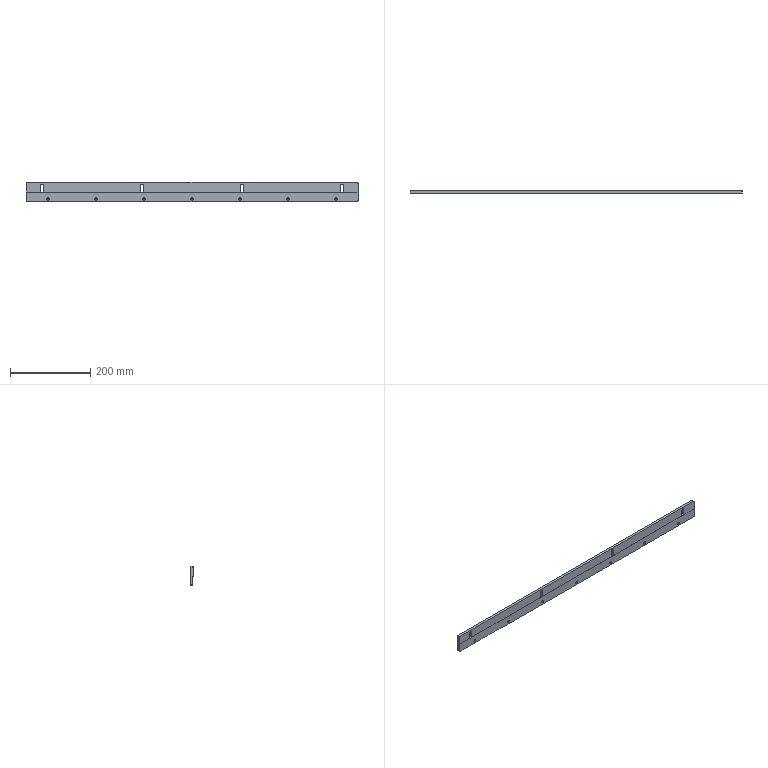Part | STEP file | BZJ-BZMM-JDKTBDYY Product限位Plate三 | 1 solid | 64 faces | box 830 x 6 x 48 mm | volume 225450 mm3 | cylinder 30 | plane 20 | cone 14 | commonest cylinder face diameters 2.5 x14 6.6 x12 4 x4